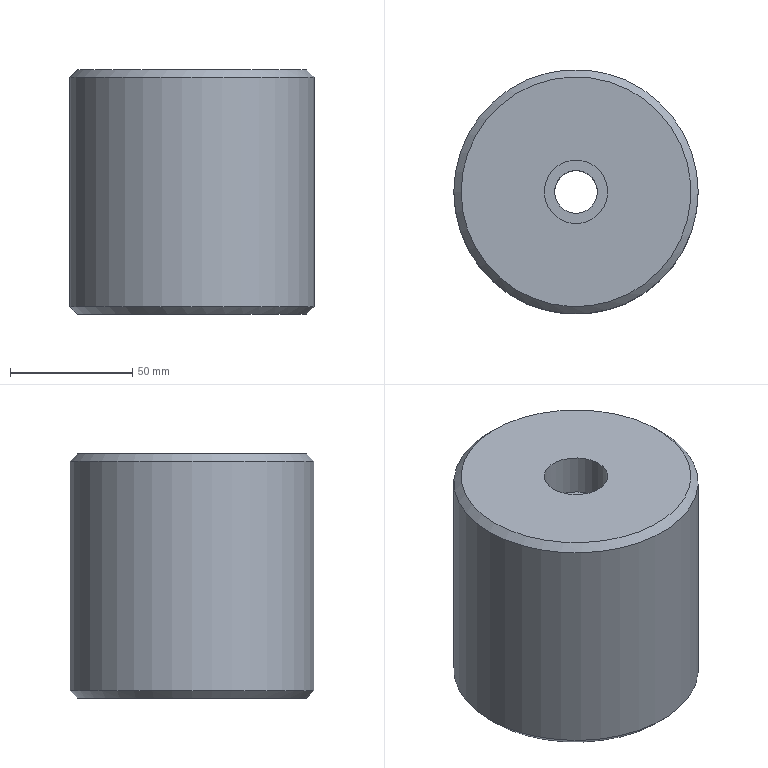Part | STEP file | solid 49 | 1 solid | 8 faces | box 100 x 100 x 100 mm | volume 753638 mm3 | plane 3 | cylinder 3 | cone 2 | commonest cylinder face diameters 17.5 x1 26 x1 100 x1